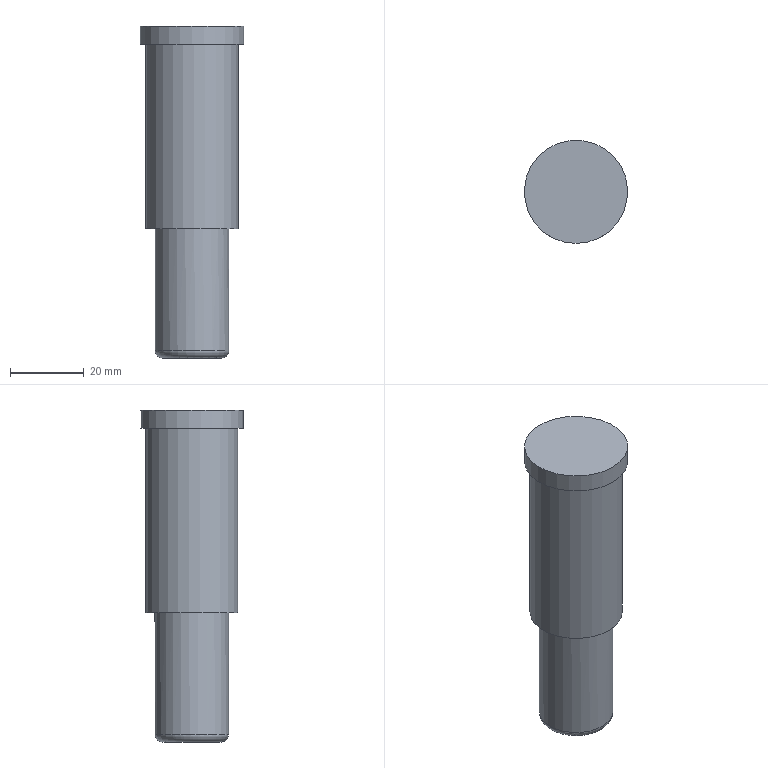Part | NX | features MAIN_BODY 2 | 1 solid | 8 faces | box 28 x 28 x 90 mm | volume 38567 mm3 | plane 4 | cylinder 3 | torus 1 | commonest cylinder face diameters 20 x1 25 x1 28 x1
STEP:
#1=CARTESIAN_POINT('',(-1274.31,439.777,74.));
#2=VERTEX_POINT('',#1);
#3=CARTESIAN_POINT('',(-1262.,441.948,74.));
#4=DIRECTION('',(0.,0.,-1.));
#5=DIRECTION('',(-0.9848,-0.1736,0.));
#6=AXIS2_PLACEMENT_3D('',#3,#4,#5);
#7=CIRCLE('',#6,12.5);
#8=EDGE_CURVE('',#2,#2,#7,.T.);
#9=ORIENTED_EDGE('',*,*,#8,.F.);
#10=EDGE_LOOP('',(#9));
#11=FACE_BOUND('',#10,.T.);
#12=CARTESIAN_POINT('',(-1274.31,439.777,124.));
#13=VERTEX_POINT('',#12);
#14=CARTESIAN_POINT('',(-1262.,441.948,124.));
#15=DIRECTION('',(0.,0.,-1.));
#16=DIRECTION('',(-0.9848,-0.1736,0.));
#17=AXIS2_PLACEMENT_3D('',#14,#15,#16);
#18=CIRCLE('',#17,12.5);
#19=EDGE_CURVE('',#13,#13,#18,.T.);
#20=ORIENTED_EDGE('',*,*,#19,.T.);
#21=EDGE_LOOP('',(#20));
#22=FACE_BOUND('',#21,.T.);
#23=CARTESIAN_POINT('',(-1262.,441.948,129.));
#24=DIRECTION('',(0.,0.,-1.));
#25=DIRECTION('',(0.9848,0.1736,0.));
#26=AXIS2_PLACEMENT_3D('',#23,#24,#25);
#27=CYLINDRICAL_SURFACE('',#26,12.5);
#28=ADVANCED_FACE('',(#11,#22),#27,.T.);
#29=CARTESIAN_POINT('',(-1271.848,440.212,74.));
#30=VERTEX_POINT('',#29);
#31=CARTESIAN_POINT('',(-1262.,441.948,74.));
#32=DIRECTION('',(0.,0.,-1.));
#33=DIRECTION('',(-0.9848,-0.1736,0.));
#34=AXIS2_PLACEMENT_3D('',#31,#32,#33);
#35=CIRCLE('',#34,10.);
#36=EDGE_CURVE('',#30,#30,#35,.T.);
#37=ORIENTED_EDGE('',*,*,#36,.F.);
#38=EDGE_LOOP('',(#37));
#39=FACE_BOUND('',#38,.T.);
#40=ORIENTED_EDGE('',*,*,#8,.T.);
#41=EDGE_LOOP('',(#40));
#42=FACE_BOUND('',#41,.T.);
#43=CARTESIAN_POINT('',(-1262.,441.948,74.));
#44=DIRECTION('',(0.,0.,1.));
#45=DIRECTION('',(-0.9848,-0.1736,0.));
#46=AXIS2_PLACEMENT_3D('',#43,#44,#45);
#47=PLANE('',#46);
#48=ADVANCED_FACE('',(#39,#42),#47,.F.);
#49=CARTESIAN_POINT('',(-1275.787,439.517,124.));
#50=VERTEX_POINT('',#49);
#51=CARTESIAN_POINT('',(-1262.,441.948,124.));
#52=DIRECTION('',(0.,0.,-1.));
#53=DIRECTION('',(-0.9848,-0.1736,0.));
#54=AXIS2_PLACEMENT_3D('',#51,#52,#53);
#55=CIRCLE('',#54,14.);
#56=EDGE_CURVE('',#50,#50,#55,.T.);
#57=ORIENTED_EDGE('',*,*,#56,.T.);
#58=EDGE_LOOP('',(#57));
#59=FACE_BOUND('',#58,.T.);
#60=ORIENTED_EDGE('',*,*,#19,.F.);
#61=EDGE_LOOP('',(#60));
#62=FACE_BOUND('',#61,.T.);
#63=CARTESIAN_POINT('',(-1262.,441.948,124.));
#64=DIRECTION('',(0.,0.,1.));
#65=DIRECTION('',(-0.9848,-0.1736,0.));
#66=AXIS2_PLACEMENT_3D('',#63,#64,#65);
#67=PLANE('',#66);
#68=ADVANCED_FACE('',(#59,#62),#67,.F.);
#69=ORIENTED_EDGE('',*,*,#56,.F.);
#70=EDGE_LOOP('',(#69));
#71=FACE_BOUND('',#70,.T.);
#72=CARTESIAN_POINT('',(-1275.787,439.517,129.));
#73=VERTEX_POINT('',#72);
#74=CARTESIAN_POINT('',(-1262.,441.948,129.));
#75=DIRECTION('',(0.,0.,-1.));
#76=DIRECTION('',(-0.9848,-0.1736,0.));
#77=AXIS2_PLACEMENT_3D('',#74,#75,#76);
#78=CIRCLE('',#77,14.);
#79=EDGE_CURVE('',#73,#73,#78,.T.);
#80=ORIENTED_EDGE('',*,*,#79,.T.);
#81=EDGE_LOOP('',(#80));
#82=FACE_BOUND('',#81,.T.);
#83=CARTESIAN_POINT('',(-1262.,441.948,125.));
#84=DIRECTION('',(0.,0.,1.));
#85=DIRECTION('',(-0.9848,-0.1736,0.));
#86=AXIS2_PLACEMENT_3D('',#83,#84,#85);
#87=CYLINDRICAL_SURFACE('',#86,14.);
#88=ADVANCED_FACE('',(#71,#82),#87,.T.);
#89=ORIENTED_EDGE('',*,*,#79,.F.);
#90=EDGE_LOOP('',(#89));
#91=FACE_BOUND('',#90,.T.);
#92=CARTESIAN_POINT('',(-1262.,441.948,129.));
#93=DIRECTION('',(0.,0.,1.));
#94=DIRECTION('',(-0.9848,-0.1736,0.));
#95=AXIS2_PLACEMENT_3D('',#92,#93,#94);
#96=PLANE('',#95);
#97=ADVANCED_FACE('',(#91),#96,.T.);
#98=CARTESIAN_POINT('',(-1252.341,444.536,41.));
#99=VERTEX_POINT('',#98);
#100=CARTESIAN_POINT('',(-1262.,441.948,41.));
#101=DIRECTION('',(0.,0.,-1.));
#102=DIRECTION('',(0.9659,0.2588,0.));
#103=AXIS2_PLACEMENT_3D('',#100,#101,#102);
#104=CIRCLE('',#103,10.);
#105=EDGE_CURVE('',#99,#99,#104,.T.);
#106=ORIENTED_EDGE('',*,*,#105,.F.);
#107=EDGE_LOOP('',(#106));
#108=FACE_BOUND('',#107,.T.);
#109=ORIENTED_EDGE('',*,*,#36,.T.);
#110=EDGE_LOOP('',(#109));
#111=FACE_BOUND('',#110,.T.);
#112=CARTESIAN_POINT('',(-1262.,441.948,49.));
#113=DIRECTION('',(0.,0.,1.));
#114=DIRECTION('',(-0.9848,-0.1736,0.));
#115=AXIS2_PLACEMENT_3D('',#112,#113,#114);
#116=CYLINDRICAL_SURFACE('',#115,10.);
#117=ADVANCED_FACE('',(#108,#111),#116,.T.);
#118=CARTESIAN_POINT('',(-1254.273,444.019,39.));
#119=VERTEX_POINT('',#118);
#120=CARTESIAN_POINT('',(-1262.,441.948,39.));
#121=DIRECTION('',(0.,0.,-1.));
#122=DIRECTION('',(0.9659,0.2588,0.));
#123=AXIS2_PLACEMENT_3D('',#120,#121,#122);
#124=CIRCLE('',#123,8.);
#125=EDGE_CURVE('',#119,#119,#124,.F.);
#126=ORIENTED_EDGE('',*,*,#125,.F.);
#127=EDGE_LOOP('',(#126));
#128=FACE_BOUND('',#127,.T.);
#129=CARTESIAN_POINT('',(-1262.,441.948,39.));
#130=DIRECTION('',(0.,0.,1.));
#131=DIRECTION('',(-0.9848,-0.1736,0.));
#132=AXIS2_PLACEMENT_3D('',#129,#130,#131);
#133=PLANE('',#132);
#134=ADVANCED_FACE('',(#128),#133,.F.);
#135=ORIENTED_EDGE('',*,*,#125,.T.);
#136=EDGE_LOOP('',(#135));
#137=FACE_BOUND('',#136,.T.);
#138=ORIENTED_EDGE('',*,*,#105,.T.);
#139=EDGE_LOOP('',(#138));
#140=FACE_BOUND('',#139,.T.);
#141=CARTESIAN_POINT('',(-1262.,441.948,41.));
#142=DIRECTION('',(0.,0.,1.));
#143=DIRECTION('',(0.9659,0.2588,0.));
#144=AXIS2_PLACEMENT_3D('',#141,#142,#143);
#145=TOROIDAL_SURFACE('',#144,8.,2.);
#146=ADVANCED_FACE('',(#137,#140),#145,.T.);
#147=CLOSED_SHELL('',(#28,#48,#68,#88,#97,#117,#134,#146));
#148=MANIFOLD_SOLID_BREP('',#147);
#149=(LENGTH_UNIT()NAMED_UNIT(*)SI_UNIT(.MILLI.,.METRE.));
#150=UNCERTAINTY_MEASURE_WITH_UNIT(LENGTH_MEASURE(0.00001),#149,'','');
#151=(NAMED_UNIT(*)PLANE_ANGLE_UNIT()SI_UNIT($,.RADIAN.));
#152=(NAMED_UNIT(*)SI_UNIT($,.STERADIAN.)SOLID_ANGLE_UNIT());
#153=(GEOMETRIC_REPRESENTATION_CONTEXT(3)GLOBAL_UNCERTAINTY_ASSIGNED_CONTEXT((#150))GLOBAL_UNIT_ASSIGNED_CONTEXT((#149,#151,#152))REPRESENTATION_CONTEXT('',''));
#154=ADVANCED_BREP_SHAPE_REPRESENTATION('',(#148),#153);